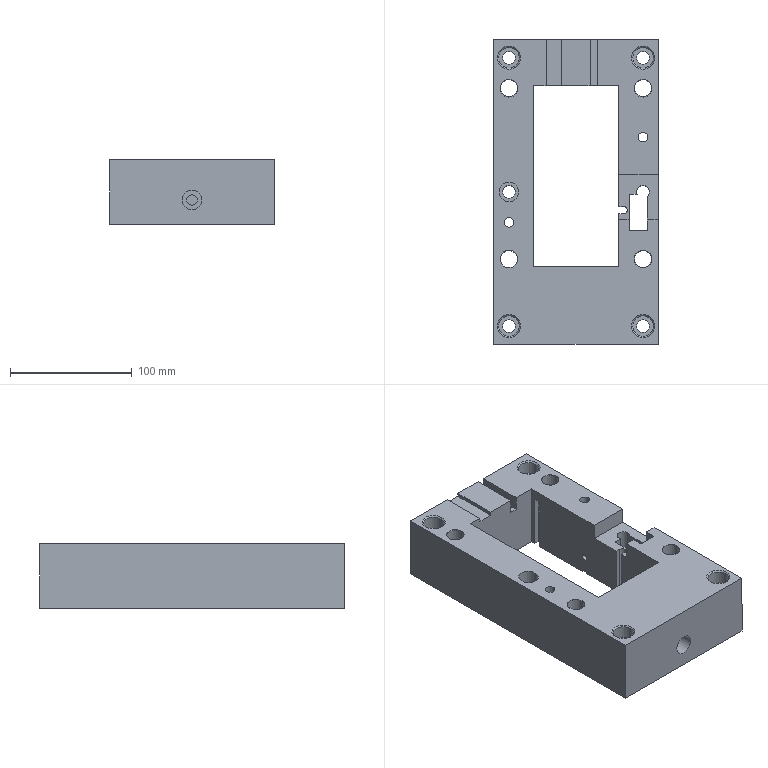Part | STEP file | KHUON BAO TREN | 1 solid | 131 faces | box 135 x 250 x 53 mm | volume 1111090 mm3 | cylinder 62 | plane 51 | cone 18 | commonest cylinder face diameters 10.5 x13 6 x8 14 x8 17 x8 18.5 x8 8 x4